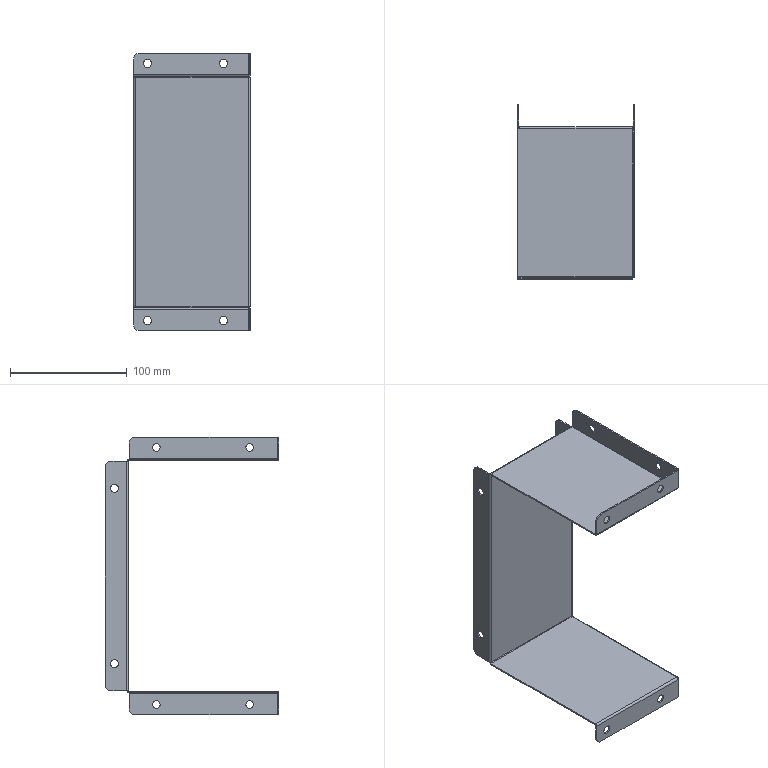Part | SolidWorks | features HoleWzd 3, EdgeFlange 2, Fillet 2, FlatPattern 1, SMBaseFlange 1, SheetMetal 1 | 1 solid | 104 faces | box 100 x 148.8 x 237.6 mm | volume 72757 mm3 | plane 52 | cylinder 48 | spline 4 | commonest cylinder face diameters 6.6 x12 7 x12 1 x8 3.4 x8 10 x8